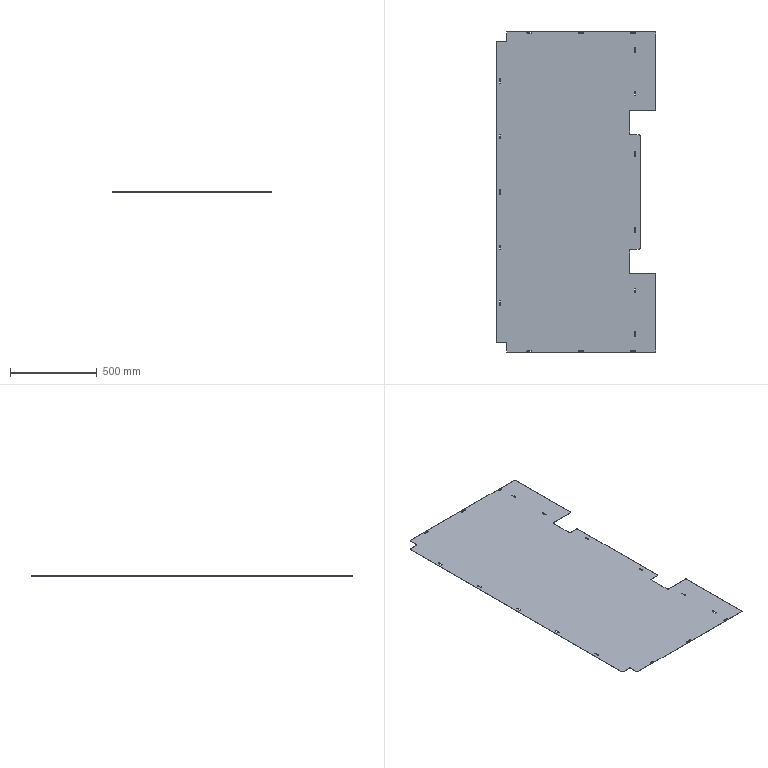Part | SolidWorks | features BaseBody 1 | 1 solid | 108 faces | box 920 x 1860 x 1.5 mm | volume 2399316 mm3 | cylinder 56 | plane 52 | commonest cylinder face diameters 7 x40 10 x16